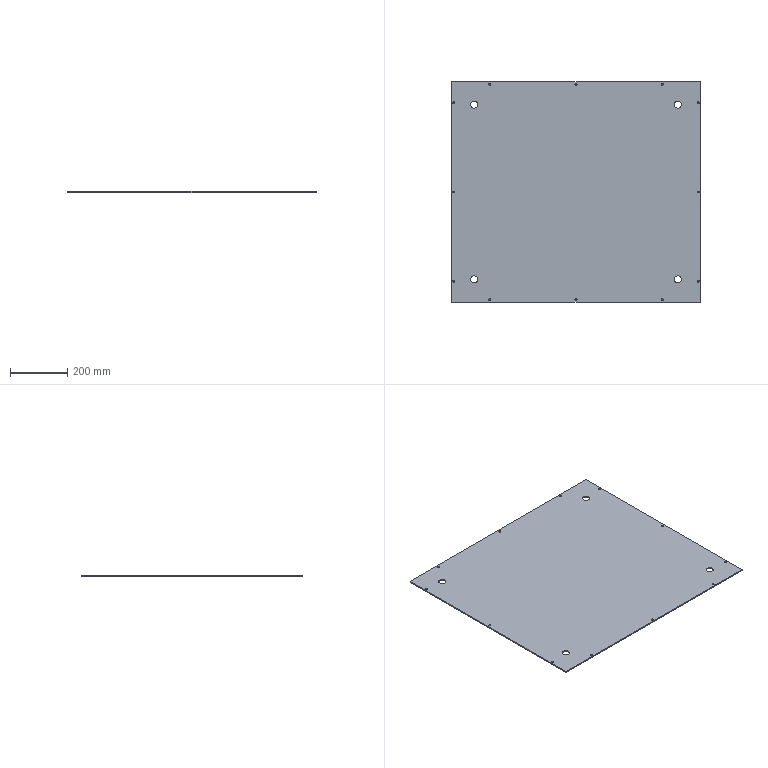Part | SolidWorks | features MirrorPattern 4, HoleWzd 2, Extrusion 1, Fillet 1, ICE 1 | 1 solid | 42 faces | box 868 x 768 x 4 mm | volume 2656781 mm3 | cylinder 36 | plane 6 | commonest cylinder face diameters 7 x24 25 x8 4 x4
STEP:
#1=CARTESIAN_POINT('',(-366.5,304.,0.));
#2=VERTEX_POINT('',#1);
#3=CARTESIAN_POINT('',(-341.5,304.,0.));
#4=VERTEX_POINT('',#3);
#5=CARTESIAN_POINT('',(-354.,304.,0.));
#6=DIRECTION('',(0.,0.,1.));
#7=DIRECTION('',(1.,0.,0.));
#8=AXIS2_PLACEMENT_3D('',#5,#6,#7);
#9=CIRCLE('',#8,12.5);
#10=EDGE_CURVE('',#2,#4,#9,.T.);
#11=ORIENTED_EDGE('',*,*,#10,.F.);
#12=CARTESIAN_POINT('',(-366.5,304.,4.));
#13=VERTEX_POINT('',#12);
#14=CARTESIAN_POINT('',(-366.5,304.,-0.001));
#15=DIRECTION('',(0.,0.,1.));
#16=VECTOR('',#15,1000.);
#17=LINE('',#14,#16);
#18=EDGE_CURVE('',#2,#13,#17,.T.);
#19=ORIENTED_EDGE('',*,*,#18,.T.);
#20=CARTESIAN_POINT('',(-341.5,304.,4.));
#21=VERTEX_POINT('',#20);
#22=CARTESIAN_POINT('',(-354.,304.,4.));
#23=DIRECTION('',(0.,0.,-1.));
#24=DIRECTION('',(1.,0.,0.));
#25=AXIS2_PLACEMENT_3D('',#22,#23,#24);
#26=CIRCLE('',#25,12.5);
#27=EDGE_CURVE('',#21,#13,#26,.T.);
#28=ORIENTED_EDGE('',*,*,#27,.F.);
#29=CARTESIAN_POINT('',(-341.5,304.,-0.001));
#30=DIRECTION('',(0.,0.,1.));
#31=VECTOR('',#30,1000.);
#32=LINE('',#29,#31);
#33=EDGE_CURVE('',#4,#21,#32,.T.);
#34=ORIENTED_EDGE('',*,*,#33,.F.);
#35=EDGE_LOOP('',(#11,#19,#28,#34));
#36=FACE_OUTER_BOUND('',#35,.T.);
#37=CARTESIAN_POINT('',(-354.,304.,-0.001));
#38=DIRECTION('',(0.,0.,1.));
#39=DIRECTION('',(1.,0.,0.));
#40=AXIS2_PLACEMENT_3D('',#37,#38,#39);
#41=CYLINDRICAL_SURFACE('',#40,12.5);
#42=ADVANCED_FACE('',(#36),#41,.F.);
#43=CARTESIAN_POINT('',(366.5,304.,0.));
#44=VERTEX_POINT('',#43);
#45=CARTESIAN_POINT('',(341.5,304.,0.));
#46=VERTEX_POINT('',#45);
#47=CARTESIAN_POINT('',(354.,304.,0.));
#48=DIRECTION('',(0.,0.,-1.));
#49=DIRECTION('',(1.,0.,0.));
#50=AXIS2_PLACEMENT_3D('',#47,#48,#49);
#51=CIRCLE('',#50,12.5);
#52=EDGE_CURVE('',#44,#46,#51,.T.);
#53=ORIENTED_EDGE('',*,*,#52,.T.);
#54=CARTESIAN_POINT('',(341.5,304.,4.));
#55=VERTEX_POINT('',#54);
#56=CARTESIAN_POINT('',(341.5,304.,-0.001));
#57=DIRECTION('',(0.,0.,1.));
#58=VECTOR('',#57,1000.);
#59=LINE('',#56,#58);
#60=EDGE_CURVE('',#46,#55,#59,.T.);
#61=ORIENTED_EDGE('',*,*,#60,.T.);
#62=CARTESIAN_POINT('',(366.5,304.,4.));
#63=VERTEX_POINT('',#62);
#64=CARTESIAN_POINT('',(354.,304.,4.));
#65=DIRECTION('',(0.,0.,1.));
#66=DIRECTION('',(-1.,0.,0.));
#67=AXIS2_PLACEMENT_3D('',#64,#65,#66);
#68=CIRCLE('',#67,12.5);
#69=EDGE_CURVE('',#55,#63,#68,.T.);
#70=ORIENTED_EDGE('',*,*,#69,.T.);
#71=CARTESIAN_POINT('',(366.5,304.,-0.001));
#72=DIRECTION('',(0.,0.,1.));
#73=VECTOR('',#72,1000.);
#74=LINE('',#71,#73);
#75=EDGE_CURVE('',#44,#63,#74,.T.);
#76=ORIENTED_EDGE('',*,*,#75,.F.);
#77=EDGE_LOOP('',(#53,#61,#70,#76));
#78=FACE_OUTER_BOUND('',#77,.T.);
#79=CARTESIAN_POINT('',(354.,304.,-0.001));
#80=DIRECTION('',(0.,0.,1.));
#81=DIRECTION('',(1.,0.,0.));
#82=AXIS2_PLACEMENT_3D('',#79,#80,#81);
#83=CYLINDRICAL_SURFACE('',#82,12.5);
#84=ADVANCED_FACE('',(#78),#83,.F.);
#85=CARTESIAN_POINT('',(341.5,-304.,0.));
#86=VERTEX_POINT('',#85);
#87=CARTESIAN_POINT('',(366.5,-304.,0.));
#88=VERTEX_POINT('',#87);
#89=CARTESIAN_POINT('',(354.,-304.,0.));
#90=DIRECTION('',(0.,0.,1.));
#91=DIRECTION('',(1.,0.,0.));
#92=AXIS2_PLACEMENT_3D('',#89,#90,#91);
#93=CIRCLE('',#92,12.5);
#94=EDGE_CURVE('',#86,#88,#93,.T.);
#95=ORIENTED_EDGE('',*,*,#94,.F.);
#96=CARTESIAN_POINT('',(341.5,-304.,4.));
#97=VERTEX_POINT('',#96);
#98=CARTESIAN_POINT('',(341.5,-304.,-0.001));
#99=DIRECTION('',(0.,0.,1.));
#100=VECTOR('',#99,1000.);
#101=LINE('',#98,#100);
#102=EDGE_CURVE('',#86,#97,#101,.T.);
#103=ORIENTED_EDGE('',*,*,#102,.T.);
#104=CARTESIAN_POINT('',(366.5,-304.,4.));
#105=VERTEX_POINT('',#104);
#106=CARTESIAN_POINT('',(354.,-304.,4.));
#107=DIRECTION('',(0.,0.,-1.));
#108=DIRECTION('',(-1.,0.,0.));
#109=AXIS2_PLACEMENT_3D('',#106,#107,#108);
#110=CIRCLE('',#109,12.5);
#111=EDGE_CURVE('',#105,#97,#110,.T.);
#112=ORIENTED_EDGE('',*,*,#111,.F.);
#113=CARTESIAN_POINT('',(366.5,-304.,-0.001));
#114=DIRECTION('',(0.,0.,1.));
#115=VECTOR('',#114,1000.);
#116=LINE('',#113,#115);
#117=EDGE_CURVE('',#88,#105,#116,.T.);
#118=ORIENTED_EDGE('',*,*,#117,.F.);
#119=EDGE_LOOP('',(#95,#103,#112,#118));
#120=FACE_OUTER_BOUND('',#119,.T.);
#121=CARTESIAN_POINT('',(354.,-304.,-0.001));
#122=DIRECTION('',(0.,0.,1.));
#123=DIRECTION('',(1.,0.,0.));
#124=AXIS2_PLACEMENT_3D('',#121,#122,#123);
#125=CYLINDRICAL_SURFACE('',#124,12.5);
#126=ADVANCED_FACE('',(#120),#125,.F.);
#127=CARTESIAN_POINT('',(-341.5,-304.,0.));
#128=VERTEX_POINT('',#127);
#129=CARTESIAN_POINT('',(-366.5,-304.,0.));
#130=VERTEX_POINT('',#129);
#131=CARTESIAN_POINT('',(-354.,-304.,0.));
#132=DIRECTION('',(0.,0.,-1.));
#133=DIRECTION('',(1.,0.,0.));
#134=AXIS2_PLACEMENT_3D('',#131,#132,#133);
#135=CIRCLE('',#134,12.5);
#136=EDGE_CURVE('',#128,#130,#135,.T.);
#137=ORIENTED_EDGE('',*,*,#136,.T.);
#138=CARTESIAN_POINT('',(-366.5,-304.,4.));
#139=VERTEX_POINT('',#138);
#140=CARTESIAN_POINT('',(-366.5,-304.,-0.001));
#141=DIRECTION('',(0.,0.,1.));
#142=VECTOR('',#141,1000.);
#143=LINE('',#140,#142);
#144=EDGE_CURVE('',#130,#139,#143,.T.);
#145=ORIENTED_EDGE('',*,*,#144,.T.);
#146=CARTESIAN_POINT('',(-341.5,-304.,4.));
#147=VERTEX_POINT('',#146);
#148=CARTESIAN_POINT('',(-354.,-304.,4.));
#149=DIRECTION('',(0.,0.,1.));
#150=DIRECTION('',(1.,0.,0.));
#151=AXIS2_PLACEMENT_3D('',#148,#149,#150);
#152=CIRCLE('',#151,12.5);
#153=EDGE_CURVE('',#139,#147,#152,.T.);
#154=ORIENTED_EDGE('',*,*,#153,.T.);
#155=CARTESIAN_POINT('',(-341.5,-304.,-0.001));
#156=DIRECTION('',(0.,0.,1.));
#157=VECTOR('',#156,1000.);
#158=LINE('',#155,#157);
#159=EDGE_CURVE('',#128,#147,#158,.T.);
#160=ORIENTED_EDGE('',*,*,#159,.F.);
#161=EDGE_LOOP('',(#137,#145,#154,#160));
#162=FACE_OUTER_BOUND('',#161,.T.);
#163=CARTESIAN_POINT('',(-354.,-304.,-0.001));
#164=DIRECTION('',(0.,0.,1.));
#165=DIRECTION('',(1.,0.,0.));
#166=AXIS2_PLACEMENT_3D('',#163,#164,#165);
#167=CYLINDRICAL_SURFACE('',#166,12.5);
#168=ADVANCED_FACE('',(#162),#167,.F.);
#169=CARTESIAN_POINT('',(-303.5,-375.,0.));
#170=VERTEX_POINT('',#169);
#171=CARTESIAN_POINT('',(-296.5,-375.,0.));
#172=VERTEX_POINT('',#171);
#173=CARTESIAN_POINT('',(-300.,-375.,0.));
#174=DIRECTION('',(0.,0.,1.));
#175=DIRECTION('',(1.,0.,0.));
#176=AXIS2_PLACEMENT_3D('',#173,#174,#175);
#177=CIRCLE('',#176,3.5);
#178=EDGE_CURVE('',#170,#172,#177,.T.);
#179=ORIENTED_EDGE('',*,*,#178,.F.);
#180=CARTESIAN_POINT('',(-303.5,-375.,4.));
#181=VERTEX_POINT('',#180);
#182=CARTESIAN_POINT('',(-303.5,-375.,4.));
#183=DIRECTION('',(0.,0.,1.));
#184=VECTOR('',#183,1000.);
#185=LINE('',#182,#184);
#186=EDGE_CURVE('',#170,#181,#185,.T.);
#187=ORIENTED_EDGE('',*,*,#186,.T.);
#188=CARTESIAN_POINT('',(-296.5,-375.,4.));
#189=VERTEX_POINT('',#188);
#190=CARTESIAN_POINT('',(-300.,-375.,4.));
#191=DIRECTION('',(0.,0.,1.));
#192=DIRECTION('',(1.,0.,0.));
#193=AXIS2_PLACEMENT_3D('',#190,#191,#192);
#194=CIRCLE('',#193,3.5);
#195=EDGE_CURVE('',#181,#189,#194,.T.);
#196=ORIENTED_EDGE('',*,*,#195,.T.);
#197=CARTESIAN_POINT('',(-296.5,-375.,4.));
#198=DIRECTION('',(0.,0.,1.));
#199=VECTOR('',#198,1000.);
#200=LINE('',#197,#199);
#201=EDGE_CURVE('',#172,#189,#200,.T.);
#202=ORIENTED_EDGE('',*,*,#201,.F.);
#203=EDGE_LOOP('',(#179,#187,#196,#202));
#204=FACE_OUTER_BOUND('',#203,.T.);
#205=CARTESIAN_POINT('',(-300.,-375.,4.));
#206=DIRECTION('',(0.,0.,1.));
#207=DIRECTION('',(1.,0.,0.));
#208=AXIS2_PLACEMENT_3D('',#205,#206,#207);
#209=CYLINDRICAL_SURFACE('',#208,3.5);
#210=ADVANCED_FACE('',(#204),#209,.F.);
#211=CARTESIAN_POINT('',(296.5,-375.,0.));
#212=VERTEX_POINT('',#211);
#213=CARTESIAN_POINT('',(303.5,-375.,0.));
#214=VERTEX_POINT('',#213);
#215=CARTESIAN_POINT('',(300.,-375.,0.));
#216=DIRECTION('',(0.,0.,1.));
#217=DIRECTION('',(1.,0.,0.));
#218=AXIS2_PLACEMENT_3D('',#215,#216,#217);
#219=CIRCLE('',#218,3.5);
#220=EDGE_CURVE('',#212,#214,#219,.T.);
#221=ORIENTED_EDGE('',*,*,#220,.F.);
#222=CARTESIAN_POINT('',(296.5,-375.,4.));
#223=VERTEX_POINT('',#222);
#224=CARTESIAN_POINT('',(296.5,-375.,4.));
#225=DIRECTION('',(0.,0.,1.));
#226=VECTOR('',#225,1000.);
#227=LINE('',#224,#226);
#228=EDGE_CURVE('',#212,#223,#227,.T.);
#229=ORIENTED_EDGE('',*,*,#228,.T.);
#230=CARTESIAN_POINT('',(303.5,-375.,4.));
#231=VERTEX_POINT('',#230);
#232=CARTESIAN_POINT('',(300.,-375.,4.));
#233=DIRECTION('',(0.,0.,1.));
#234=DIRECTION('',(1.,0.,0.));
#235=AXIS2_PLACEMENT_3D('',#232,#233,#234);
#236=CIRCLE('',#235,3.5);
#237=EDGE_CURVE('',#223,#231,#236,.T.);
#238=ORIENTED_EDGE('',*,*,#237,.T.);
#239=CARTESIAN_POINT('',(303.5,-375.,4.));
#240=DIRECTION('',(0.,0.,1.));
#241=VECTOR('',#240,1000.);
#242=LINE('',#239,#241);
#243=EDGE_CURVE('',#214,#231,#242,.T.);
#244=ORIENTED_EDGE('',*,*,#243,.F.);
#245=EDGE_LOOP('',(#221,#229,#238,#244));
#246=FACE_OUTER_BOUND('',#245,.T.);
#247=CARTESIAN_POINT('',(300.,-375.,4.));
#248=DIRECTION('',(0.,0.,1.));
#249=DIRECTION('',(1.,0.,0.));
#250=AXIS2_PLACEMENT_3D('',#247,#248,#249);
#251=CYLINDRICAL_SURFACE('',#250,3.5);
#252=ADVANCED_FACE('',(#246),#251,.F.);
#253=CARTESIAN_POINT('',(-3.5,-375.,0.));
#254=VERTEX_POINT('',#253);
#255=CARTESIAN_POINT('',(3.5,-375.,0.));
#256=VERTEX_POINT('',#255);
#257=CARTESIAN_POINT('',(0.,-375.,0.));
#258=DIRECTION('',(0.,0.,1.));
#259=DIRECTION('',(1.,0.,0.));
#260=AXIS2_PLACEMENT_3D('',#257,#258,#259);
#261=CIRCLE('',#260,3.5);
#262=EDGE_CURVE('',#254,#256,#261,.T.);
#263=ORIENTED_EDGE('',*,*,#262,.F.);
#264=CARTESIAN_POINT('',(-3.5,-375.,4.));
#265=VERTEX_POINT('',#264);
#266=CARTESIAN_POINT('',(-3.5,-375.,4.));
#267=DIRECTION('',(0.,0.,1.));
#268=VECTOR('',#267,1000.);
#269=LINE('',#266,#268);
#270=EDGE_CURVE('',#254,#265,#269,.T.);
#271=ORIENTED_EDGE('',*,*,#270,.T.);
#272=CARTESIAN_POINT('',(3.5,-375.,4.));
#273=VERTEX_POINT('',#272);
#274=CARTESIAN_POINT('',(0.,-375.,4.));
#275=DIRECTION('',(0.,0.,1.));
#276=DIRECTION('',(1.,0.,0.));
#277=AXIS2_PLACEMENT_3D('',#274,#275,#276);
#278=CIRCLE('',#277,3.5);
#279=EDGE_CURVE('',#265,#273,#278,.T.);
#280=ORIENTED_EDGE('',*,*,#279,.T.);
#281=CARTESIAN_POINT('',(3.5,-375.,4.));
#282=DIRECTION('',(0.,0.,1.));
#283=VECTOR('',#282,1000.);
#284=LINE('',#281,#283);
#285=EDGE_CURVE('',#256,#273,#284,.T.);
#286=ORIENTED_EDGE('',*,*,#285,.F.);
#287=EDGE_LOOP('',(#263,#271,#280,#286));
#288=FACE_OUTER_BOUND('',#287,.T.);
#289=CARTESIAN_POINT('',(0.,-375.,4.));
#290=DIRECTION('',(0.,0.,1.));
#291=DIRECTION('',(1.,0.,0.));
#292=AXIS2_PLACEMENT_3D('',#289,#290,#291);
#293=CYLINDRICAL_SURFACE('',#292,3.5);
#294=ADVANCED_FACE('',(#288),#293,.F.);
#295=CARTESIAN_POINT('',(-303.5,375.,0.));
#296=VERTEX_POINT('',#295);
#297=CARTESIAN_POINT('',(-296.5,375.,0.));
#298=VERTEX_POINT('',#297);
#299=CARTESIAN_POINT('',(-300.,375.,0.));
#300=DIRECTION('',(0.,0.,1.));
#301=DIRECTION('',(1.,0.,0.));
#302=AXIS2_PLACEMENT_3D('',#299,#300,#301);
#303=CIRCLE('',#302,3.5);
#304=EDGE_CURVE('',#296,#298,#303,.T.);
#305=ORIENTED_EDGE('',*,*,#304,.F.);
#306=CARTESIAN_POINT('',(-303.5,375.,4.));
#307=VERTEX_POINT('',#306);
#308=CARTESIAN_POINT('',(-303.5,375.,4.));
#309=DIRECTION('',(0.,0.,1.));
#310=VECTOR('',#309,1000.);
#311=LINE('',#308,#310);
#312=EDGE_CURVE('',#296,#307,#311,.T.);
#313=ORIENTED_EDGE('',*,*,#312,.T.);
#314=CARTESIAN_POINT('',(-296.5,375.,4.));
#315=VERTEX_POINT('',#314);
#316=CARTESIAN_POINT('',(-300.,375.,4.));
#317=DIRECTION('',(0.,0.,1.));
#318=DIRECTION('',(1.,0.,0.));
#319=AXIS2_PLACEMENT_3D('',#316,#317,#318);
#320=CIRCLE('',#319,3.5);
#321=EDGE_CURVE('',#307,#315,#320,.T.);
#322=ORIENTED_EDGE('',*,*,#321,.T.);
#323=CARTESIAN_POINT('',(-296.5,375.,4.));
#324=DIRECTION('',(0.,0.,1.));
#325=VECTOR('',#324,1000.);
#326=LINE('',#323,#325);
#327=EDGE_CURVE('',#298,#315,#326,.T.);
#328=ORIENTED_EDGE('',*,*,#327,.F.);
#329=EDGE_LOOP('',(#305,#313,#322,#328));
#330=FACE_OUTER_BOUND('',#329,.T.);
#331=CARTESIAN_POINT('',(-300.,375.,4.));
#332=DIRECTION('',(0.,0.,1.));
#333=DIRECTION('',(1.,0.,0.));
#334=AXIS2_PLACEMENT_3D('',#331,#332,#333);
#335=CYLINDRICAL_SURFACE('',#334,3.5);
#336=ADVANCED_FACE('',(#330),#335,.F.);
#337=CARTESIAN_POINT('',(296.5,375.,0.));
#338=VERTEX_POINT('',#337);
#339=CARTESIAN_POINT('',(303.5,375.,0.));
#340=VERTEX_POINT('',#339);
#341=CARTESIAN_POINT('',(300.,375.,0.));
#342=DIRECTION('',(0.,0.,1.));
#343=DIRECTION('',(1.,0.,0.));
#344=AXIS2_PLACEMENT_3D('',#341,#342,#343);
#345=CIRCLE('',#344,3.5);
#346=EDGE_CURVE('',#338,#340,#345,.T.);
#347=ORIENTED_EDGE('',*,*,#346,.F.);
#348=CARTESIAN_POINT('',(296.5,375.,4.));
#349=VERTEX_POINT('',#348);
#350=CARTESIAN_POINT('',(296.5,375.,4.));
#351=DIRECTION('',(0.,0.,1.));
#352=VECTOR('',#351,1000.);
#353=LINE('',#350,#352);
#354=EDGE_CURVE('',#338,#349,#353,.T.);
#355=ORIENTED_EDGE('',*,*,#354,.T.);
#356=CARTESIAN_POINT('',(303.5,375.,4.));
#357=VERTEX_POINT('',#356);
#358=CARTESIAN_POINT('',(300.,375.,4.));
#359=DIRECTION('',(0.,0.,1.));
#360=DIRECTION('',(1.,0.,0.));
#361=AXIS2_PLACEMENT_3D('',#358,#359,#360);
#362=CIRCLE('',#361,3.5);
#363=EDGE_CURVE('',#349,#357,#362,.T.);
#364=ORIENTED_EDGE('',*,*,#363,.T.);
#365=CARTESIAN_POINT('',(303.5,375.,4.));
#366=DIRECTION('',(0.,0.,1.));
#367=VECTOR('',#366,1000.);
#368=LINE('',#365,#367);
#369=EDGE_CURVE('',#340,#357,#368,.T.);
#370=ORIENTED_EDGE('',*,*,#369,.F.);
#371=EDGE_LOOP('',(#347,#355,#364,#370));
#372=FACE_OUTER_BOUND('',#371,.T.);
#373=CARTESIAN_POINT('',(300.,375.,4.));
#374=DIRECTION('',(0.,0.,1.));
#375=DIRECTION('',(1.,0.,0.));
#376=AXIS2_PLACEMENT_3D('',#373,#374,#375);
#377=CYLINDRICAL_SURFACE('',#376,3.5);
#378=ADVANCED_FACE('',(#372),#377,.F.);
#379=CARTESIAN_POINT('',(-3.5,375.,0.));
#380=VERTEX_POINT('',#379);
#381=CARTESIAN_POINT('',(3.5,375.,0.));
#382=VERTEX_POINT('',#381);
#383=CARTESIAN_POINT('',(0.,375.,0.));
#384=DIRECTION('',(0.,0.,1.));
#385=DIRECTION('',(1.,0.,0.));
#386=AXIS2_PLACEMENT_3D('',#383,#384,#385);
#387=CIRCLE('',#386,3.5);
#388=EDGE_CURVE('',#380,#382,#387,.T.);
#389=ORIENTED_EDGE('',*,*,#388,.F.);
#390=CARTESIAN_POINT('',(-3.5,375.,4.));
#391=VERTEX_POINT('',#390);
#392=CARTESIAN_POINT('',(-3.5,375.,4.));
#393=DIRECTION('',(0.,0.,1.));
#394=VECTOR('',#393,1000.);
#395=LINE('',#392,#394);
#396=EDGE_CURVE('',#380,#391,#395,.T.);
#397=ORIENTED_EDGE('',*,*,#396,.T.);
#398=CARTESIAN_POINT('',(3.5,375.,4.));
#399=VERTEX_POINT('',#398);
#400=CARTESIAN_POINT('',(0.,375.,4.));
#401=DIRECTION('',(0.,0.,1.));
#402=DIRECTION('',(1.,0.,0.));
#403=AXIS2_PLACEMENT_3D('',#400,#401,#402);
#404=CIRCLE('',#403,3.5);
#405=EDGE_CURVE('',#391,#399,#404,.T.);
#406=ORIENTED_EDGE('',*,*,#405,.T.);
#407=CARTESIAN_POINT('',(3.5,375.,4.));
#408=DIRECTION('',(0.,0.,1.));
#409=VECTOR('',#408,1000.);
#410=LINE('',#407,#409);
#411=EDGE_CURVE('',#382,#399,#410,.T.);
#412=ORIENTED_EDGE('',*,*,#411,.F.);
#413=EDGE_LOOP('',(#389,#397,#406,#412));
#414=FACE_OUTER_BOUND('',#413,.T.);
#415=CARTESIAN_POINT('',(0.,375.,4.));
#416=DIRECTION('',(0.,0.,1.));
#417=DIRECTION('',(1.,0.,0.));
#418=AXIS2_PLACEMENT_3D('',#415,#416,#417);
#419=CYLINDRICAL_SURFACE('',#418,3.5);
#420=ADVANCED_FACE('',(#414),#419,.F.);
#421=CARTESIAN_POINT('',(421.5,310.,0.));
#422=VERTEX_POINT('',#421);
#423=CARTESIAN_POINT('',(428.5,310.,0.));
#424=VERTEX_POINT('',#423);
#425=CARTESIAN_POINT('',(425.,310.,0.));
#426=DIRECTION('',(0.,0.,1.));
#427=DIRECTION('',(1.,0.,0.));
#428=AXIS2_PLACEMENT_3D('',#425,#426,#427);
#429=CIRCLE('',#428,3.5);
#430=EDGE_CURVE('',#422,#424,#429,.T.);
#431=ORIENTED_EDGE('',*,*,#430,.F.);
#432=CARTESIAN_POINT('',(421.5,310.,4.));
#433=VERTEX_POINT('',#432);
#434=CARTESIAN_POINT('',(421.5,310.,4.));
#435=DIRECTION('',(0.,0.,1.));
#436=VECTOR('',#435,1000.);
#437=LINE('',#434,#436);
#438=EDGE_CURVE('',#422,#433,#437,.T.);
#439=ORIENTED_EDGE('',*,*,#438,.T.);
#440=CARTESIAN_POINT('',(428.5,310.,4.));
#441=VERTEX_POINT('',#440);
#442=CARTESIAN_POINT('',(425.,310.,4.));
#443=DIRECTION('',(0.,0.,1.));
#444=DIRECTION('',(1.,0.,0.));
#445=AXIS2_PLACEMENT_3D('',#442,#443,#444);
#446=CIRCLE('',#445,3.5);
#447=EDGE_CURVE('',#433,#441,#446,.T.);
#448=ORIENTED_EDGE('',*,*,#447,.T.);
#449=CARTESIAN_POINT('',(428.5,310.,4.));
#450=DIRECTION('',(0.,0.,1.));
#451=VECTOR('',#450,1000.);
#452=LINE('',#449,#451);
#453=EDGE_CURVE('',#424,#441,#452,.T.);
#454=ORIENTED_EDGE('',*,*,#453,.F.);
#455=EDGE_LOOP('',(#431,#439,#448,#454));
#456=FACE_OUTER_BOUND('',#455,.T.);
#457=CARTESIAN_POINT('',(425.,310.,4.));
#458=DIRECTION('',(0.,0.,1.));
#459=DIRECTION('',(1.,0.,0.));
#460=AXIS2_PLACEMENT_3D('',#457,#458,#459);
#461=CYLINDRICAL_SURFACE('',#460,3.5);
#462=ADVANCED_FACE('',(#456),#461,.F.);
#463=CARTESIAN_POINT('',(421.5,-310.,0.));
#464=VERTEX_POINT('',#463);
#465=CARTESIAN_POINT('',(428.5,-310.,0.));
#466=VERTEX_POINT('',#465);
#467=CARTESIAN_POINT('',(425.,-310.,0.));
#468=DIRECTION('',(0.,0.,1.));
#469=DIRECTION('',(1.,0.,0.));
#470=AXIS2_PLACEMENT_3D('',#467,#468,#469);
#471=CIRCLE('',#470,3.5);
#472=EDGE_CURVE('',#464,#466,#471,.T.);
#473=ORIENTED_EDGE('',*,*,#472,.F.);
#474=CARTESIAN_POINT('',(421.5,-310.,4.));
#475=VERTEX_POINT('',#474);
#476=CARTESIAN_POINT('',(421.5,-310.,4.));
#477=DIRECTION('',(0.,0.,1.));
#478=VECTOR('',#477,1000.);
#479=LINE('',#476,#478);
#480=EDGE_CURVE('',#464,#475,#479,.T.);
#481=ORIENTED_EDGE('',*,*,#480,.T.);
#482=CARTESIAN_POINT('',(428.5,-310.,4.));
#483=VERTEX_POINT('',#482);
#484=CARTESIAN_POINT('',(425.,-310.,4.));
#485=DIRECTION('',(0.,0.,1.));
#486=DIRECTION('',(1.,0.,0.));
#487=AXIS2_PLACEMENT_3D('',#484,#485,#486);
#488=CIRCLE('',#487,3.5);
#489=EDGE_CURVE('',#475,#483,#488,.T.);
#490=ORIENTED_EDGE('',*,*,#489,.T.);
#491=CARTESIAN_POINT('',(428.5,-310.,4.));
#492=DIRECTION('',(0.,0.,1.));
#493=VECTOR('',#492,1000.);
#494=LINE('',#491,#493);
#495=EDGE_CURVE('',#466,#483,#494,.T.);
#496=ORIENTED_EDGE('',*,*,#495,.F.);
#497=EDGE_LOOP('',(#473,#481,#490,#496));
#498=FACE_OUTER_BOUND('',#497,.T.);
#499=CARTESIAN_POINT('',(425.,-310.,4.));
#500=DIRECTION('',(0.,0.,1.));
#501=DIRECTION('',(1.,0.,0.));
#502=AXIS2_PLACEMENT_3D('',#499,#500,#501);
#503=CYLINDRICAL_SURFACE('',#502,3.5);
#504=ADVANCED_FACE('',(#498),#503,.F.);
#505=CARTESIAN_POINT('',(421.5,0.,0.));
#506=VERTEX_POINT('',#505);
#507=CARTESIAN_POINT('',(428.5,0.,0.));
#508=VERTEX_POINT('',#507);
#509=CARTESIAN_POINT('',(425.,0.,0.));
#510=DIRECTION('',(0.,0.,1.));
#511=DIRECTION('',(1.,0.,0.));
#512=AXIS2_PLACEMENT_3D('',#509,#510,#511);
#513=CIRCLE('',#512,3.5);
#514=EDGE_CURVE('',#506,#508,#513,.T.);
#515=ORIENTED_EDGE('',*,*,#514,.F.);
#516=CARTESIAN_POINT('',(421.5,0.,4.));
#517=VERTEX_POINT('',#516);
#518=CARTESIAN_POINT('',(421.5,0.,4.));
#519=DIRECTION('',(0.,0.,1.));
#520=VECTOR('',#519,1000.);
#521=LINE('',#518,#520);
#522=EDGE_CURVE('',#506,#517,#521,.T.);
#523=ORIENTED_EDGE('',*,*,#522,.T.);
#524=CARTESIAN_POINT('',(428.5,0.,4.));
#525=VERTEX_POINT('',#524);
#526=CARTESIAN_POINT('',(425.,0.,4.));
#527=DIRECTION('',(0.,0.,1.));
#528=DIRECTION('',(1.,0.,0.));
#529=AXIS2_PLACEMENT_3D('',#526,#527,#528);
#530=CIRCLE('',#529,3.5);
#531=EDGE_CURVE('',#517,#525,#530,.T.);
#532=ORIENTED_EDGE('',*,*,#531,.T.);
#533=CARTESIAN_POINT('',(428.5,0.,4.));
#534=DIRECTION('',(0.,0.,1.));
#535=VECTOR('',#534,1000.);
#536=LINE('',#533,#535);
#537=EDGE_CURVE('',#508,#525,#536,.T.);
#538=ORIENTED_EDGE('',*,*,#537,.F.);
#539=EDGE_LOOP('',(#515,#523,#532,#538));
#540=FACE_OUTER_BOUND('',#539,.T.);
#541=CARTESIAN_POINT('',(425.,0.,4.));
#542=DIRECTION('',(0.,0.,1.));
#543=DIRECTION('',(1.,0.,0.));
#544=AXIS2_PLACEMENT_3D('',#541,#542,#543);
#545=CYLINDRICAL_SURFACE('',#544,3.5);
#546=ADVANCED_FACE('',(#540),#545,.F.);
#547=CARTESIAN_POINT('',(-428.5,310.,0.));
#548=VERTEX_POINT('',#547);
#549=CARTESIAN_POINT('',(-421.5,310.,0.));
#550=VERTEX_POINT('',#549);
#551=CARTESIAN_POINT('',(-425.,310.,0.));
#552=DIRECTION('',(0.,0.,1.));
#553=DIRECTION('',(1.,0.,0.));
#554=AXIS2_PLACEMENT_3D('',#551,#552,#553);
#555=CIRCLE('',#554,3.5);
#556=EDGE_CURVE('',#548,#550,#555,.T.);
#557=ORIENTED_EDGE('',*,*,#556,.F.);
#558=CARTESIAN_POINT('',(-428.5,310.,4.));
#559=VERTEX_POINT('',#558);
#560=CARTESIAN_POINT('',(-428.5,310.,4.));
#561=DIRECTION('',(0.,0.,1.));
#562=VECTOR('',#561,1000.);
#563=LINE('',#560,#562);
#564=EDGE_CURVE('',#548,#559,#563,.T.);
#565=ORIENTED_EDGE('',*,*,#564,.T.);
#566=CARTESIAN_POINT('',(-421.5,310.,4.));
#567=VERTEX_POINT('',#566);
#568=CARTESIAN_POINT('',(-425.,310.,4.));
#569=DIRECTION('',(0.,0.,1.));
#570=DIRECTION('',(1.,0.,0.));
#571=AXIS2_PLACEMENT_3D('',#568,#569,#570);
#572=CIRCLE('',#571,3.5);
#573=EDGE_CURVE('',#559,#567,#572,.T.);
#574=ORIENTED_EDGE('',*,*,#573,.T.);
#575=CARTESIAN_POINT('',(-421.5,310.,4.));
#576=DIRECTION('',(0.,0.,1.));
#577=VECTOR('',#576,1000.);
#578=LINE('',#575,#577);
#579=EDGE_CURVE('',#550,#567,#578,.T.);
#580=ORIENTED_EDGE('',*,*,#579,.F.);
#581=EDGE_LOOP('',(#557,#565,#574,#580));
#582=FACE_OUTER_BOUND('',#581,.T.);
#583=CARTESIAN_POINT('',(-425.,310.,4.));
#584=DIRECTION('',(0.,0.,1.));
#585=DIRECTION('',(1.,0.,0.));
#586=AXIS2_PLACEMENT_3D('',#583,#584,#585);
#587=CYLINDRICAL_SURFACE('',#586,3.5);
#588=ADVANCED_FACE('',(#582),#587,.F.);
#589=CARTESIAN_POINT('',(-428.5,-310.,0.));
#590=VERTEX_POINT('',#589);
#591=CARTESIAN_POINT('',(-421.5,-310.,0.));
#592=VERTEX_POINT('',#591);
#593=CARTESIAN_POINT('',(-425.,-310.,0.));
#594=DIRECTION('',(0.,0.,1.));
#595=DIRECTION('',(1.,0.,0.));
#596=AXIS2_PLACEMENT_3D('',#593,#594,#595);
#597=CIRCLE('',#596,3.5);
#598=EDGE_CURVE('',#590,#592,#597,.T.);
#599=ORIENTED_EDGE('',*,*,#598,.F.);
#600=CARTESIAN_POINT('',(-428.5,-310.,4.));
#601=VERTEX_POINT('',#600);
#602=CARTESIAN_POINT('',(-428.5,-310.,4.));
#603=DIRECTION('',(0.,0.,1.));
#604=VECTOR('',#603,1000.);
#605=LINE('',#602,#604);
#606=EDGE_CURVE('',#590,#601,#605,.T.);
#607=ORIENTED_EDGE('',*,*,#606,.T.);
#608=CARTESIAN_POINT('',(-421.5,-310.,4.));
#609=VERTEX_POINT('',#608);
#610=CARTESIAN_POINT('',(-425.,-310.,4.));
#611=DIRECTION('',(0.,0.,1.));
#612=DIRECTION('',(1.,0.,0.));
#613=AXIS2_PLACEMENT_3D('',#610,#611,#612);
#614=CIRCLE('',#613,3.5);
#615=EDGE_CURVE('',#601,#609,#614,.T.);
#616=ORIENTED_EDGE('',*,*,#615,.T.);
#617=CARTESIAN_POINT('',(-421.5,-310.,4.));
#618=DIRECTION('',(0.,0.,1.));
#619=VECTOR('',#618,1000.);
#620=LINE('',#617,#619);
#621=EDGE_CURVE('',#592,#609,#620,.T.);
#622=ORIENTED_EDGE('',*,*,#621,.F.);
#623=EDGE_LOOP('',(#599,#607,#616,#622));
#624=FACE_OUTER_BOUND('',#623,.T.);
#625=CARTESIAN_POINT('',(-425.,-310.,4.));
#626=DIRECTION('',(0.,0.,1.));
#627=DIRECTION('',(1.,0.,0.));
#628=AXIS2_PLACEMENT_3D('',#625,#626,#627);
#629=CYLINDRICAL_SURFACE('',#628,3.5);
#630=ADVANCED_FACE('',(#624),#629,.F.);
#631=CARTESIAN_POINT('',(-428.5,0.,0.));
#632=VERTEX_POINT('',#631);
#633=CARTESIAN_POINT('',(-421.5,0.,0.));
#634=VERTEX_POINT('',#633);
#635=CARTESIAN_POINT('',(-425.,0.,0.));
#636=DIRECTION('',(0.,0.,1.));
#637=DIRECTION('',(1.,0.,0.));
#638=AXIS2_PLACEMENT_3D('',#635,#636,#637);
#639=CIRCLE('',#638,3.5);
#640=EDGE_CURVE('',#632,#634,#639,.T.);
#641=ORIENTED_EDGE('',*,*,#640,.F.);
#642=CARTESIAN_POINT('',(-428.5,0.,4.));
#643=VERTEX_POINT('',#642);
#644=CARTESIAN_POINT('',(-428.5,0.,4.));
#645=DIRECTION('',(0.,0.,1.));
#646=VECTOR('',#645,1000.);
#647=LINE('',#644,#646);
#648=EDGE_CURVE('',#632,#643,#647,.T.);
#649=ORIENTED_EDGE('',*,*,#648,.T.);
#650=CARTESIAN_POINT('',(-421.5,0.,4.));
#651=VERTEX_POINT('',#650);
#652=CARTESIAN_POINT('',(-425.,0.,4.));
#653=DIRECTION('',(0.,0.,1.));
#654=DIRECTION('',(1.,0.,0.));
#655=AXIS2_PLACEMENT_3D('',#652,#653,#654);
#656=CIRCLE('',#655,3.5);
#657=EDGE_CURVE('',#643,#651,#656,.T.);
#658=ORIENTED_EDGE('',*,*,#657,.T.);
#659=CARTESIAN_POINT('',(-421.5,0.,4.));
#660=DIRECTION('',(0.,0.,1.));
#661=VECTOR('',#660,1000.);
#662=LINE('',#659,#661);
#663=EDGE_CURVE('',#634,#651,#662,.T.);
#664=ORIENTED_EDGE('',*,*,#663,.F.);
#665=EDGE_LOOP('',(#641,#649,#658,#664));
#666=FACE_OUTER_BOUND('',#665,.T.);
#667=CARTESIAN_POINT('',(-425.,0.,4.));
#668=DIRECTION('',(0.,0.,1.));
#669=DIRECTION('',(1.,0.,0.));
#670=AXIS2_PLACEMENT_3D('',#667,#668,#669);
#671=CYLINDRICAL_SURFACE('',#670,3.5);
#672=ADVANCED_FACE('',(#666),#671,.F.);
#673=CARTESIAN_POINT('',(-434.,382.,0.));
#674=VERTEX_POINT('',#673);
#675=CARTESIAN_POINT('',(-434.,-382.,0.));
#676=VERTEX_POINT('',#675);
#677=CARTESIAN_POINT('',(-434.,-384.,0.));
#678=DIRECTION('',(0.,-1.,0.));
#679=VECTOR('',#678,1000.);
#680=LINE('',#677,#679);
#681=EDGE_CURVE('',#674,#676,#680,.T.);
#682=ORIENTED_EDGE('',*,*,#681,.T.);
#683=CARTESIAN_POINT('',(-434.,-382.,4.));
#684=VERTEX_POINT('',#683);
#685=CARTESIAN_POINT('',(-434.,-382.,4.));
#686=DIRECTION('',(0.,0.,1.));
#687=VECTOR('',#686,1000.);
#688=LINE('',#685,#687);
#689=EDGE_CURVE('',#676,#684,#688,.T.);
#690=ORIENTED_EDGE('',*,*,#689,.T.);
#691=CARTESIAN_POINT('',(-434.,382.,4.));
#692=VERTEX_POINT('',#691);
#693=CARTESIAN_POINT('',(-434.,-384.,4.));
#694=DIRECTION('',(0.,-1.,0.));
#695=VECTOR('',#694,1000.);
#696=LINE('',#693,#695);
#697=EDGE_CURVE('',#692,#684,#696,.T.);
#698=ORIENTED_EDGE('',*,*,#697,.F.);
#699=CARTESIAN_POINT('',(-434.,382.,4.));
#700=DIRECTION('',(0.,0.,-1.));
#701=VECTOR('',#700,1000.);
#702=LINE('',#699,#701);
#703=EDGE_CURVE('',#692,#674,#702,.T.);
#704=ORIENTED_EDGE('',*,*,#703,.T.);
#705=EDGE_LOOP('',(#682,#690,#698,#704));
#706=FACE_OUTER_BOUND('',#705,.T.);
#707=CARTESIAN_POINT('',(-434.,-384.,4.));
#708=DIRECTION('',(1.,0.,0.));
#709=DIRECTION('',(0.,0.,-1.));
#710=AXIS2_PLACEMENT_3D('',#707,#708,#709);
#711=PLANE('',#710);
#712=ADVANCED_FACE('',(#706),#711,.F.);
#713=CARTESIAN_POINT('',(-432.,-384.,0.));
#714=VERTEX_POINT('',#713);
#715=CARTESIAN_POINT('',(432.,-384.,0.));
#716=VERTEX_POINT('',#715);
#717=CARTESIAN_POINT('',(434.,-384.,0.));
#718=DIRECTION('',(1.,0.,0.));
#719=VECTOR('',#718,1000.);
#720=LINE('',#717,#719);
#721=EDGE_CURVE('',#714,#716,#720,.T.);
#722=ORIENTED_EDGE('',*,*,#721,.T.);
#723=CARTESIAN_POINT('',(432.,-384.,4.));
#724=VERTEX_POINT('',#723);
#725=CARTESIAN_POINT('',(432.,-384.,4.));
#726=DIRECTION('',(0.,0.,1.));
#727=VECTOR('',#726,1000.);
#728=LINE('',#725,#727);
#729=EDGE_CURVE('',#716,#724,#728,.T.);
#730=ORIENTED_EDGE('',*,*,#729,.T.);
#731=CARTESIAN_POINT('',(-432.,-384.,4.));
#732=VERTEX_POINT('',#731);
#733=CARTESIAN_POINT('',(434.,-384.,4.));
#734=DIRECTION('',(1.,0.,0.));
#735=VECTOR('',#734,1000.);
#736=LINE('',#733,#735);
#737=EDGE_CURVE('',#732,#724,#736,.T.);
#738=ORIENTED_EDGE('',*,*,#737,.F.);
#739=CARTESIAN_POINT('',(-432.,-384.,4.));
#740=DIRECTION('',(0.,0.,-1.));
#741=VECTOR('',#740,1000.);
#742=LINE('',#739,#741);
#743=EDGE_CURVE('',#732,#714,#742,.T.);
#744=ORIENTED_EDGE('',*,*,#743,.T.);
#745=EDGE_LOOP('',(#722,#730,#738,#744));
#746=FACE_OUTER_BOUND('',#745,.T.);
#747=CARTESIAN_POINT('',(434.,-384.,4.));
#748=DIRECTION('',(0.,1.,0.));
#749=DIRECTION('',(-1.,0.,0.));
#750=AXIS2_PLACEMENT_3D('',#747,#748,#749);
#751=PLANE('',#750);
#752=ADVANCED_FACE('',(#746),#751,.F.);
#753=CARTESIAN_POINT('',(434.,-382.,0.));
#754=VERTEX_POINT('',#753);
#755=CARTESIAN_POINT('',(434.,382.,0.));
#756=VERTEX_POINT('',#755);
#757=CARTESIAN_POINT('',(434.,-384.,0.));
#758=DIRECTION('',(0.,1.,0.));
#759=VECTOR('',#758,1000.);
#760=LINE('',#757,#759);
#761=EDGE_CURVE('',#754,#756,#760,.T.);
#762=ORIENTED_EDGE('',*,*,#761,.T.);
#763=CARTESIAN_POINT('',(434.,382.,4.));
#764=VERTEX_POINT('',#763);
#765=CARTESIAN_POINT('',(434.,382.,4.));
#766=DIRECTION('',(0.,0.,1.));
#767=VECTOR('',#766,1000.);
#768=LINE('',#765,#767);
#769=EDGE_CURVE('',#756,#764,#768,.T.);
#770=ORIENTED_EDGE('',*,*,#769,.T.);
#771=CARTESIAN_POINT('',(434.,-382.,4.));
#772=VERTEX_POINT('',#771);
#773=CARTESIAN_POINT('',(434.,-384.,4.));
#774=DIRECTION('',(0.,1.,0.));
#775=VECTOR('',#774,1000.);
#776=LINE('',#773,#775);
#777=EDGE_CURVE('',#772,#764,#776,.T.);
#778=ORIENTED_EDGE('',*,*,#777,.F.);
#779=CARTESIAN_POINT('',(434.,-382.,4.));
#780=DIRECTION('',(0.,0.,-1.));
#781=VECTOR('',#780,1000.);
#782=LINE('',#779,#781);
#783=EDGE_CURVE('',#772,#754,#782,.T.);
#784=ORIENTED_EDGE('',*,*,#783,.T.);
#785=EDGE_LOOP('',(#762,#770,#778,#784));
#786=FACE_OUTER_BOUND('',#785,.T.);
#787=CARTESIAN_POINT('',(434.,-384.,4.));
#788=DIRECTION('',(-1.,0.,0.));
#789=DIRECTION('',(0.,-1.,0.));
#790=AXIS2_PLACEMENT_3D('',#787,#788,#789);
#791=PLANE('',#790);
#792=ADVANCED_FACE('',(#786),#791,.F.);
#793=CARTESIAN_POINT('',(432.,384.,4.));
#794=VERTEX_POINT('',#793);
#795=CARTESIAN_POINT('',(-432.,384.,4.));
#796=VERTEX_POINT('',#795);
#797=CARTESIAN_POINT('',(434.,384.,4.));
#798=DIRECTION('',(-1.,0.,0.));
#799=VECTOR('',#798,1000.);
#800=LINE('',#797,#799);
#801=EDGE_CURVE('',#794,#796,#800,.T.);
#802=ORIENTED_EDGE('',*,*,#801,.F.);
#803=CARTESIAN_POINT('',(432.,384.,0.));
#804=VERTEX_POINT('',#803);
#805=CARTESIAN_POINT('',(432.,384.,4.));
#806=DIRECTION('',(0.,0.,-1.));
#807=VECTOR('',#806,1000.);
#808=LINE('',#805,#807);
#809=EDGE_CURVE('',#794,#804,#808,.T.);
#810=ORIENTED_EDGE('',*,*,#809,.T.);
#811=CARTESIAN_POINT('',(-432.,384.,0.));
#812=VERTEX_POINT('',#811);
#813=CARTESIAN_POINT('',(434.,384.,0.));
#814=DIRECTION('',(-1.,0.,0.));
#815=VECTOR('',#814,1000.);
#816=LINE('',#813,#815);
#817=EDGE_CURVE('',#804,#812,#816,.T.);
#818=ORIENTED_EDGE('',*,*,#817,.T.);
#819=CARTESIAN_POINT('',(-432.,384.,4.));
#820=DIRECTION('',(0.,0.,1.));
#821=VECTOR('',#820,1000.);
#822=LINE('',#819,#821);
#823=EDGE_CURVE('',#812,#796,#822,.T.);
#824=ORIENTED_EDGE('',*,*,#823,.T.);
#825=EDGE_LOOP('',(#802,#810,#818,#824));
#826=FACE_OUTER_BOUND('',#825,.T.);
#827=CARTESIAN_POINT('',(434.,384.,4.));
#828=DIRECTION('',(0.,-1.,0.));
#829=DIRECTION('',(1.,0.,0.));
#830=AXIS2_PLACEMENT_3D('',#827,#828,#829);
#831=PLANE('',#830);
#832=ADVANCED_FACE('',(#826),#831,.F.);
#833=ORIENTED_EDGE('',*,*,#27,.T.);
#834=CARTESIAN_POINT('',(-354.,304.,4.));
#835=DIRECTION('',(0.,0.,-1.));
#836=DIRECTION('',(1.,0.,0.));
#837=AXIS2_PLACEMENT_3D('',#834,#835,#836);
#838=CIRCLE('',#837,12.5);
#839=EDGE_CURVE('',#13,#21,#838,.T.);
#840=ORIENTED_EDGE('',*,*,#839,.T.);
#841=EDGE_LOOP('',(#833,#840));
#842=FACE_BOUND('',#841,.T.);
#843=CARTESIAN_POINT('',(354.,304.,4.));
#844=DIRECTION('',(0.,0.,1.));
#845=DIRECTION('',(-1.,0.,0.));
#846=AXIS2_PLACEMENT_3D('',#843,#844,#845);
#847=CIRCLE('',#846,12.5);
#848=EDGE_CURVE('',#63,#55,#847,.T.);
#849=ORIENTED_EDGE('',*,*,#848,.F.);
#850=ORIENTED_EDGE('',*,*,#69,.F.);
#851=EDGE_LOOP('',(#849,#850));
#852=FACE_BOUND('',#851,.T.);
#853=ORIENTED_EDGE('',*,*,#111,.T.);
#854=CARTESIAN_POINT('',(354.,-304.,4.));
#855=DIRECTION('',(0.,0.,-1.));
#856=DIRECTION('',(-1.,0.,0.));
#857=AXIS2_PLACEMENT_3D('',#854,#855,#856);
#858=CIRCLE('',#857,12.5);
#859=EDGE_CURVE('',#97,#105,#858,.T.);
#860=ORIENTED_EDGE('',*,*,#859,.T.);
#861=EDGE_LOOP('',(#853,#860));
#862=FACE_BOUND('',#861,.T.);
#863=CARTESIAN_POINT('',(-354.,-304.,4.));
#864=DIRECTION('',(0.,0.,1.));
#865=DIRECTION('',(1.,0.,0.));
#866=AXIS2_PLACEMENT_3D('',#863,#864,#865);
#867=CIRCLE('',#866,12.5);
#868=EDGE_CURVE('',#147,#139,#867,.T.);
#869=ORIENTED_EDGE('',*,*,#868,.F.);
#870=ORIENTED_EDGE('',*,*,#153,.F.);
#871=EDGE_LOOP('',(#869,#870));
#872=FACE_BOUND('',#871,.T.);
#873=CARTESIAN_POINT('',(-300.,-375.,4.));
#874=DIRECTION('',(0.,0.,1.));
#875=DIRECTION('',(1.,0.,0.));
#876=AXIS2_PLACEMENT_3D('',#873,#874,#875);
#877=CIRCLE('',#876,3.5);
#878=EDGE_CURVE('',#189,#181,#877,.T.);
#879=ORIENTED_EDGE('',*,*,#878,.F.);
#880=ORIENTED_EDGE('',*,*,#195,.F.);
#881=EDGE_LOOP('',(#879,#880));
#882=FACE_BOUND('',#881,.T.);
#883=CARTESIAN_POINT('',(300.,-375.,4.));
#884=DIRECTION('',(0.,0.,1.));
#885=DIRECTION('',(1.,0.,0.));
#886=AXIS2_PLACEMENT_3D('',#883,#884,#885);
#887=CIRCLE('',#886,3.5);
#888=EDGE_CURVE('',#231,#223,#887,.T.);
#889=ORIENTED_EDGE('',*,*,#888,.F.);
#890=ORIENTED_EDGE('',*,*,#237,.F.);
#891=EDGE_LOOP('',(#889,#890));
#892=FACE_BOUND('',#891,.T.);
#893=CARTESIAN_POINT('',(0.,-375.,4.));
#894=DIRECTION('',(0.,0.,1.));
#895=DIRECTION('',(1.,0.,0.));
#896=AXIS2_PLACEMENT_3D('',#893,#894,#895);
#897=CIRCLE('',#896,3.5);
#898=EDGE_CURVE('',#273,#265,#897,.T.);
#899=ORIENTED_EDGE('',*,*,#898,.F.);
#900=ORIENTED_EDGE('',*,*,#279,.F.);
#901=EDGE_LOOP('',(#899,#900));
#902=FACE_BOUND('',#901,.T.);
#903=CARTESIAN_POINT('',(-300.,375.,4.));
#904=DIRECTION('',(0.,0.,1.));
#905=DIRECTION('',(1.,0.,0.));
#906=AXIS2_PLACEMENT_3D('',#903,#904,#905);
#907=CIRCLE('',#906,3.5);
#908=EDGE_CURVE('',#315,#307,#907,.T.);
#909=ORIENTED_EDGE('',*,*,#908,.F.);
#910=ORIENTED_EDGE('',*,*,#321,.F.);
#911=EDGE_LOOP('',(#909,#910));
#912=FACE_BOUND('',#911,.T.);
#913=CARTESIAN_POINT('',(300.,375.,4.));
#914=DIRECTION('',(0.,0.,1.));
#915=DIRECTION('',(1.,0.,0.));
#916=AXIS2_PLACEMENT_3D('',#913,#914,#915);
#917=CIRCLE('',#916,3.5);
#918=EDGE_CURVE('',#357,#349,#917,.T.);
#919=ORIENTED_EDGE('',*,*,#918,.F.);
#920=ORIENTED_EDGE('',*,*,#363,.F.);
#921=EDGE_LOOP('',(#919,#920));
#922=FACE_BOUND('',#921,.T.);
#923=CARTESIAN_POINT('',(0.,375.,4.));
#924=DIRECTION('',(0.,0.,1.));
#925=DIRECTION('',(1.,0.,0.));
#926=AXIS2_PLACEMENT_3D('',#923,#924,#925);
#927=CIRCLE('',#926,3.5);
#928=EDGE_CURVE('',#399,#391,#927,.T.);
#929=ORIENTED_EDGE('',*,*,#928,.F.);
#930=ORIENTED_EDGE('',*,*,#405,.F.);
#931=EDGE_LOOP('',(#929,#930));
#932=FACE_BOUND('',#931,.T.);
#933=CARTESIAN_POINT('',(425.,310.,4.));
#934=DIRECTION('',(0.,0.,1.));
#935=DIRECTION('',(1.,0.,0.));
#936=AXIS2_PLACEMENT_3D('',#933,#934,#935);
#937=CIRCLE('',#936,3.5);
#938=EDGE_CURVE('',#441,#433,#937,.T.);
#939=ORIENTED_EDGE('',*,*,#938,.F.);
#940=ORIENTED_EDGE('',*,*,#447,.F.);
#941=EDGE_LOOP('',(#939,#940));
#942=FACE_BOUND('',#941,.T.);
#943=CARTESIAN_POINT('',(425.,-310.,4.));
#944=DIRECTION('',(0.,0.,1.));
#945=DIRECTION('',(1.,0.,0.));
#946=AXIS2_PLACEMENT_3D('',#943,#944,#945);
#947=CIRCLE('',#946,3.5);
#948=EDGE_CURVE('',#483,#475,#947,.T.);
#949=ORIENTED_EDGE('',*,*,#948,.F.);
#950=ORIENTED_EDGE('',*,*,#489,.F.);
#951=EDGE_LOOP('',(#949,#950));
#952=FACE_BOUND('',#951,.T.);
#953=CARTESIAN_POINT('',(425.,0.,4.));
#954=DIRECTION('',(0.,0.,1.));
#955=DIRECTION('',(1.,0.,0.));
#956=AXIS2_PLACEMENT_3D('',#953,#954,#955);
#957=CIRCLE('',#956,3.5);
#958=EDGE_CURVE('',#525,#517,#957,.T.);
#959=ORIENTED_EDGE('',*,*,#958,.F.);
#960=ORIENTED_EDGE('',*,*,#531,.F.);
#961=EDGE_LOOP('',(#959,#960));
#962=FACE_BOUND('',#961,.T.);
#963=CARTESIAN_POINT('',(-425.,310.,4.));
#964=DIRECTION('',(0.,0.,1.));
#965=DIRECTION('',(1.,0.,0.));
#966=AXIS2_PLACEMENT_3D('',#963,#964,#965);
#967=CIRCLE('',#966,3.5);
#968=EDGE_CURVE('',#567,#559,#967,.T.);
#969=ORIENTED_EDGE('',*,*,#968,.F.);
#970=ORIENTED_EDGE('',*,*,#573,.F.);
#971=EDGE_LOOP('',(#969,#970));
#972=FACE_BOUND('',#971,.T.);
#973=CARTESIAN_POINT('',(-425.,-310.,4.));
#974=DIRECTION('',(0.,0.,1.));
#975=DIRECTION('',(1.,0.,0.));
#976=AXIS2_PLACEMENT_3D('',#973,#974,#975);
#977=CIRCLE('',#976,3.5);
#978=EDGE_CURVE('',#609,#601,#977,.T.);
#979=ORIENTED_EDGE('',*,*,#978,.F.);
#980=ORIENTED_EDGE('',*,*,#615,.F.);
#981=EDGE_LOOP('',(#979,#980));
#982=FACE_BOUND('',#981,.T.);
#983=CARTESIAN_POINT('',(-425.,0.,4.));
#984=DIRECTION('',(0.,0.,1.));
#985=DIRECTION('',(1.,0.,0.));
#986=AXIS2_PLACEMENT_3D('',#983,#984,#985);
#987=CIRCLE('',#986,3.5);
#988=EDGE_CURVE('',#651,#643,#987,.T.);
#989=ORIENTED_EDGE('',*,*,#988,.F.);
#990=ORIENTED_EDGE('',*,*,#657,.F.);
#991=EDGE_LOOP('',(#989,#990));
#992=FACE_BOUND('',#991,.T.);
#993=ORIENTED_EDGE('',*,*,#777,.T.);
#994=CARTESIAN_POINT('',(432.,382.,4.));
#995=DIRECTION('',(0.,0.,1.));
#996=DIRECTION('',(1.,0.,0.));
#997=AXIS2_PLACEMENT_3D('',#994,#995,#996);
#998=CIRCLE('',#997,2.);
#999=EDGE_CURVE('',#764,#794,#998,.T.);
#1000=ORIENTED_EDGE('',*,*,#999,.T.);
#1001=ORIENTED_EDGE('',*,*,#801,.T.);
#1002=CARTESIAN_POINT('',(-432.,382.,4.));
#1003=DIRECTION('',(0.,0.,1.));
#1004=DIRECTION('',(1.,0.,0.));
#1005=AXIS2_PLACEMENT_3D('',#1002,#1003,#1004);
#1006=CIRCLE('',#1005,2.);
#1007=EDGE_CURVE('',#796,#692,#1006,.T.);
#1008=ORIENTED_EDGE('',*,*,#1007,.T.);
#1009=ORIENTED_EDGE('',*,*,#697,.T.);
#1010=CARTESIAN_POINT('',(-432.,-382.,4.));
#1011=DIRECTION('',(0.,0.,1.));
#1012=DIRECTION('',(1.,0.,0.));
#1013=AXIS2_PLACEMENT_3D('',#1010,#1011,#1012);
#1014=CIRCLE('',#1013,2.);
#1015=EDGE_CURVE('',#684,#732,#1014,.T.);
#1016=ORIENTED_EDGE('',*,*,#1015,.T.);
#1017=ORIENTED_EDGE('',*,*,#737,.T.);
#1018=CARTESIAN_POINT('',(432.,-382.,4.));
#1019=DIRECTION('',(0.,0.,1.));
#1020=DIRECTION('',(1.,0.,0.));
#1021=AXIS2_PLACEMENT_3D('',#1018,#1019,#1020);
#1022=CIRCLE('',#1021,2.);
#1023=EDGE_CURVE('',#724,#772,#1022,.T.);
#1024=ORIENTED_EDGE('',*,*,#1023,.T.);
#1025=EDGE_LOOP('',(#993,#1000,#1001,#1008,#1009,#1016,#1017,#1024));
#1026=FACE_OUTER_BOUND('',#1025,.T.);
#1027=CARTESIAN_POINT('',(0.,0.,4.));
#1028=DIRECTION('',(0.,0.,1.));
#1029=DIRECTION('',(1.,0.,0.));
#1030=AXIS2_PLACEMENT_3D('',#1027,#1028,#1029);
#1031=PLANE('',#1030);
#1032=ADVANCED_FACE('',(#842,#852,#862,#872,#882,#892,#902,#912,#922,#932,#942,#952,#962,#972,#982,#992,#1026),#1031,.T.);
#1033=CARTESIAN_POINT('',(-354.,304.,0.));
#1034=DIRECTION('',(0.,0.,1.));
#1035=DIRECTION('',(1.,0.,0.));
#1036=AXIS2_PLACEMENT_3D('',#1033,#1034,#1035);
#1037=CIRCLE('',#1036,12.5);
#1038=EDGE_CURVE('',#4,#2,#1037,.T.);
#1039=ORIENTED_EDGE('',*,*,#1038,.T.);
#1040=ORIENTED_EDGE('',*,*,#10,.T.);
#1041=EDGE_LOOP('',(#1039,#1040));
#1042=FACE_BOUND('',#1041,.T.);
#1043=ORIENTED_EDGE('',*,*,#52,.F.);
#1044=CARTESIAN_POINT('',(354.,304.,0.));
#1045=DIRECTION('',(0.,0.,-1.));
#1046=DIRECTION('',(1.,0.,0.));
#1047=AXIS2_PLACEMENT_3D('',#1044,#1045,#1046);
#1048=CIRCLE('',#1047,12.5);
#1049=EDGE_CURVE('',#46,#44,#1048,.T.);
#1050=ORIENTED_EDGE('',*,*,#1049,.F.);
#1051=EDGE_LOOP('',(#1043,#1050));
#1052=FACE_BOUND('',#1051,.T.);
#1053=CARTESIAN_POINT('',(354.,-304.,0.));
#1054=DIRECTION('',(0.,0.,1.));
#1055=DIRECTION('',(1.,0.,0.));
#1056=AXIS2_PLACEMENT_3D('',#1053,#1054,#1055);
#1057=CIRCLE('',#1056,12.5);
#1058=EDGE_CURVE('',#88,#86,#1057,.T.);
#1059=ORIENTED_EDGE('',*,*,#1058,.T.);
#1060=ORIENTED_EDGE('',*,*,#94,.T.);
#1061=EDGE_LOOP('',(#1059,#1060));
#1062=FACE_BOUND('',#1061,.T.);
#1063=ORIENTED_EDGE('',*,*,#136,.F.);
#1064=CARTESIAN_POINT('',(-354.,-304.,0.));
#1065=DIRECTION('',(0.,0.,-1.));
#1066=DIRECTION('',(1.,0.,0.));
#1067=AXIS2_PLACEMENT_3D('',#1064,#1065,#1066);
#1068=CIRCLE('',#1067,12.5);
#1069=EDGE_CURVE('',#130,#128,#1068,.T.);
#1070=ORIENTED_EDGE('',*,*,#1069,.F.);
#1071=EDGE_LOOP('',(#1063,#1070));
#1072=FACE_BOUND('',#1071,.T.);
#1073=CARTESIAN_POINT('',(-300.,-375.,0.));
#1074=DIRECTION('',(0.,0.,1.));
#1075=DIRECTION('',(1.,0.,0.));
#1076=AXIS2_PLACEMENT_3D('',#1073,#1074,#1075);
#1077=CIRCLE('',#1076,3.5);
#1078=EDGE_CURVE('',#172,#170,#1077,.T.);
#1079=ORIENTED_EDGE('',*,*,#1078,.T.);
#1080=ORIENTED_EDGE('',*,*,#178,.T.);
#1081=EDGE_LOOP('',(#1079,#1080));
#1082=FACE_BOUND('',#1081,.T.);
#1083=CARTESIAN_POINT('',(300.,-375.,0.));
#1084=DIRECTION('',(0.,0.,1.));
#1085=DIRECTION('',(1.,0.,0.));
#1086=AXIS2_PLACEMENT_3D('',#1083,#1084,#1085);
#1087=CIRCLE('',#1086,3.5);
#1088=EDGE_CURVE('',#214,#212,#1087,.T.);
#1089=ORIENTED_EDGE('',*,*,#1088,.T.);
#1090=ORIENTED_EDGE('',*,*,#220,.T.);
#1091=EDGE_LOOP('',(#1089,#1090));
#1092=FACE_BOUND('',#1091,.T.);
#1093=CARTESIAN_POINT('',(0.,-375.,0.));
#1094=DIRECTION('',(0.,0.,1.));
#1095=DIRECTION('',(1.,0.,0.));
#1096=AXIS2_PLACEMENT_3D('',#1093,#1094,#1095);
#1097=CIRCLE('',#1096,3.5);
#1098=EDGE_CURVE('',#256,#254,#1097,.T.);
#1099=ORIENTED_EDGE('',*,*,#1098,.T.);
#1100=ORIENTED_EDGE('',*,*,#262,.T.);
#1101=EDGE_LOOP('',(#1099,#1100));
#1102=FACE_BOUND('',#1101,.T.);
#1103=CARTESIAN_POINT('',(-300.,375.,0.));
#1104=DIRECTION('',(0.,0.,1.));
#1105=DIRECTION('',(1.,0.,0.));
#1106=AXIS2_PLACEMENT_3D('',#1103,#1104,#1105);
#1107=CIRCLE('',#1106,3.5);
#1108=EDGE_CURVE('',#298,#296,#1107,.T.);
#1109=ORIENTED_EDGE('',*,*,#1108,.T.);
#1110=ORIENTED_EDGE('',*,*,#304,.T.);
#1111=EDGE_LOOP('',(#1109,#1110));
#1112=FACE_BOUND('',#1111,.T.);
#1113=CARTESIAN_POINT('',(300.,375.,0.));
#1114=DIRECTION('',(0.,0.,1.));
#1115=DIRECTION('',(1.,0.,0.));
#1116=AXIS2_PLACEMENT_3D('',#1113,#1114,#1115);
#1117=CIRCLE('',#1116,3.5);
#1118=EDGE_CURVE('',#340,#338,#1117,.T.);
#1119=ORIENTED_EDGE('',*,*,#1118,.T.);
#1120=ORIENTED_EDGE('',*,*,#346,.T.);
#1121=EDGE_LOOP('',(#1119,#1120));
#1122=FACE_BOUND('',#1121,.T.);
#1123=CARTESIAN_POINT('',(0.,375.,0.));
#1124=DIRECTION('',(0.,0.,1.));
#1125=DIRECTION('',(1.,0.,0.));
#1126=AXIS2_PLACEMENT_3D('',#1123,#1124,#1125);
#1127=CIRCLE('',#1126,3.5);
#1128=EDGE_CURVE('',#382,#380,#1127,.T.);
#1129=ORIENTED_EDGE('',*,*,#1128,.T.);
#1130=ORIENTED_EDGE('',*,*,#388,.T.);
#1131=EDGE_LOOP('',(#1129,#1130));
#1132=FACE_BOUND('',#1131,.T.);
#1133=CARTESIAN_POINT('',(425.,310.,0.));
#1134=DIRECTION('',(0.,0.,1.));
#1135=DIRECTION('',(1.,0.,0.));
#1136=AXIS2_PLACEMENT_3D('',#1133,#1134,#1135);
#1137=CIRCLE('',#1136,3.5);
#1138=EDGE_CURVE('',#424,#422,#1137,.T.);
#1139=ORIENTED_EDGE('',*,*,#1138,.T.);
#1140=ORIENTED_EDGE('',*,*,#430,.T.);
#1141=EDGE_LOOP('',(#1139,#1140));
#1142=FACE_BOUND('',#1141,.T.);
#1143=CARTESIAN_POINT('',(425.,-310.,0.));
#1144=DIRECTION('',(0.,0.,1.));
#1145=DIRECTION('',(1.,0.,0.));
#1146=AXIS2_PLACEMENT_3D('',#1143,#1144,#1145);
#1147=CIRCLE('',#1146,3.5);
#1148=EDGE_CURVE('',#466,#464,#1147,.T.);
#1149=ORIENTED_EDGE('',*,*,#1148,.T.);
#1150=ORIENTED_EDGE('',*,*,#472,.T.);
#1151=EDGE_LOOP('',(#1149,#1150));
#1152=FACE_BOUND('',#1151,.T.);
#1153=CARTESIAN_POINT('',(425.,0.,0.));
#1154=DIRECTION('',(0.,0.,1.));
#1155=DIRECTION('',(1.,0.,0.));
#1156=AXIS2_PLACEMENT_3D('',#1153,#1154,#1155);
#1157=CIRCLE('',#1156,3.5);
#1158=EDGE_CURVE('',#508,#506,#1157,.T.);
#1159=ORIENTED_EDGE('',*,*,#1158,.T.);
#1160=ORIENTED_EDGE('',*,*,#514,.T.);
#1161=EDGE_LOOP('',(#1159,#1160));
#1162=FACE_BOUND('',#1161,.T.);
#1163=CARTESIAN_POINT('',(-425.,310.,0.));
#1164=DIRECTION('',(0.,0.,1.));
#1165=DIRECTION('',(1.,0.,0.));
#1166=AXIS2_PLACEMENT_3D('',#1163,#1164,#1165);
#1167=CIRCLE('',#1166,3.5);
#1168=EDGE_CURVE('',#550,#548,#1167,.T.);
#1169=ORIENTED_EDGE('',*,*,#1168,.T.);
#1170=ORIENTED_EDGE('',*,*,#556,.T.);
#1171=EDGE_LOOP('',(#1169,#1170));
#1172=FACE_BOUND('',#1171,.T.);
#1173=CARTESIAN_POINT('',(-425.,-310.,0.));
#1174=DIRECTION('',(0.,0.,1.));
#1175=DIRECTION('',(1.,0.,0.));
#1176=AXIS2_PLACEMENT_3D('',#1173,#1174,#1175);
#1177=CIRCLE('',#1176,3.5);
#1178=EDGE_CURVE('',#592,#590,#1177,.T.);
#1179=ORIENTED_EDGE('',*,*,#1178,.T.);
#1180=ORIENTED_EDGE('',*,*,#598,.T.);
#1181=EDGE_LOOP('',(#1179,#1180));
#1182=FACE_BOUND('',#1181,.T.);
#1183=CARTESIAN_POINT('',(-425.,0.,0.));
#1184=DIRECTION('',(0.,0.,1.));
#1185=DIRECTION('',(1.,0.,0.));
#1186=AXIS2_PLACEMENT_3D('',#1183,#1184,#1185);
#1187=CIRCLE('',#1186,3.5);
#1188=EDGE_CURVE('',#634,#632,#1187,.T.);
#1189=ORIENTED_EDGE('',*,*,#1188,.T.);
#1190=ORIENTED_EDGE('',*,*,#640,.T.);
#1191=EDGE_LOOP('',(#1189,#1190));
#1192=FACE_BOUND('',#1191,.T.);
#1193=ORIENTED_EDGE('',*,*,#817,.F.);
#1194=CARTESIAN_POINT('',(432.,382.,0.));
#1195=DIRECTION('',(0.,0.,-1.));
#1196=DIRECTION('',(1.,0.,0.));
#1197=AXIS2_PLACEMENT_3D('',#1194,#1195,#1196);
#1198=CIRCLE('',#1197,2.);
#1199=EDGE_CURVE('',#804,#756,#1198,.T.);
#1200=ORIENTED_EDGE('',*,*,#1199,.T.);
#1201=ORIENTED_EDGE('',*,*,#761,.F.);
#1202=CARTESIAN_POINT('',(432.,-382.,0.));
#1203=DIRECTION('',(0.,0.,-1.));
#1204=DIRECTION('',(1.,0.,0.));
#1205=AXIS2_PLACEMENT_3D('',#1202,#1203,#1204);
#1206=CIRCLE('',#1205,2.);
#1207=EDGE_CURVE('',#754,#716,#1206,.T.);
#1208=ORIENTED_EDGE('',*,*,#1207,.T.);
#1209=ORIENTED_EDGE('',*,*,#721,.F.);
#1210=CARTESIAN_POINT('',(-432.,-382.,0.));
#1211=DIRECTION('',(0.,0.,-1.));
#1212=DIRECTION('',(1.,0.,0.));
#1213=AXIS2_PLACEMENT_3D('',#1210,#1211,#1212);
#1214=CIRCLE('',#1213,2.);
#1215=EDGE_CURVE('',#714,#676,#1214,.T.);
#1216=ORIENTED_EDGE('',*,*,#1215,.T.);
#1217=ORIENTED_EDGE('',*,*,#681,.F.);
#1218=CARTESIAN_POINT('',(-432.,382.,0.));
#1219=DIRECTION('',(0.,0.,-1.));
#1220=DIRECTION('',(1.,0.,0.));
#1221=AXIS2_PLACEMENT_3D('',#1218,#1219,#1220);
#1222=CIRCLE('',#1221,2.);
#1223=EDGE_CURVE('',#674,#812,#1222,.T.);
#1224=ORIENTED_EDGE('',*,*,#1223,.T.);
#1225=EDGE_LOOP('',(#1193,#1200,#1201,#1208,#1209,#1216,#1217,#1224));
#1226=FACE_OUTER_BOUND('',#1225,.T.);
#1227=CARTESIAN_POINT('',(0.,0.,0.));
#1228=DIRECTION('',(0.,0.,1.));
#1229=DIRECTION('',(1.,0.,0.));
#1230=AXIS2_PLACEMENT_3D('',#1227,#1228,#1229);
#1231=PLANE('',#1230);
#1232=ADVANCED_FACE('',(#1042,#1052,#1062,#1072,#1082,#1092,#1102,#1112,#1122,#1132,#1142,#1152,#1162,#1172,#1182,#1192,#1226),#1231,.F.);
#1233=ORIENTED_EDGE('',*,*,#999,.F.);
#1234=ORIENTED_EDGE('',*,*,#769,.F.);
#1235=ORIENTED_EDGE('',*,*,#1199,.F.);
#1236=ORIENTED_EDGE('',*,*,#809,.F.);
#1237=EDGE_LOOP('',(#1233,#1234,#1235,#1236));
#1238=FACE_OUTER_BOUND('',#1237,.T.);
#1239=CARTESIAN_POINT('',(432.,382.,4.));
#1240=DIRECTION('',(0.,0.,-1.));
#1241=DIRECTION('',(-1.,0.,0.));
#1242=AXIS2_PLACEMENT_3D('',#1239,#1240,#1241);
#1243=CYLINDRICAL_SURFACE('',#1242,2.);
#1244=ADVANCED_FACE('',(#1238),#1243,.T.);
#1245=ORIENTED_EDGE('',*,*,#1023,.F.);
#1246=ORIENTED_EDGE('',*,*,#729,.F.);
#1247=ORIENTED_EDGE('',*,*,#1207,.F.);
#1248=ORIENTED_EDGE('',*,*,#783,.F.);
#1249=EDGE_LOOP('',(#1245,#1246,#1247,#1248));
#1250=FACE_OUTER_BOUND('',#1249,.T.);
#1251=CARTESIAN_POINT('',(432.,-382.,4.));
#1252=DIRECTION('',(0.,0.,-1.));
#1253=DIRECTION('',(-1.,0.,0.));
#1254=AXIS2_PLACEMENT_3D('',#1251,#1252,#1253);
#1255=CYLINDRICAL_SURFACE('',#1254,2.);
#1256=ADVANCED_FACE('',(#1250),#1255,.T.);
#1257=ORIENTED_EDGE('',*,*,#1015,.F.);
#1258=ORIENTED_EDGE('',*,*,#689,.F.);
#1259=ORIENTED_EDGE('',*,*,#1215,.F.);
#1260=ORIENTED_EDGE('',*,*,#743,.F.);
#1261=EDGE_LOOP('',(#1257,#1258,#1259,#1260));
#1262=FACE_OUTER_BOUND('',#1261,.T.);
#1263=CARTESIAN_POINT('',(-432.,-382.,4.));
#1264=DIRECTION('',(0.,0.,-1.));
#1265=DIRECTION('',(-1.,0.,0.));
#1266=AXIS2_PLACEMENT_3D('',#1263,#1264,#1265);
#1267=CYLINDRICAL_SURFACE('',#1266,2.);
#1268=ADVANCED_FACE('',(#1262),#1267,.T.);
#1269=ORIENTED_EDGE('',*,*,#1007,.F.);
#1270=ORIENTED_EDGE('',*,*,#823,.F.);
#1271=ORIENTED_EDGE('',*,*,#1223,.F.);
#1272=ORIENTED_EDGE('',*,*,#703,.F.);
#1273=EDGE_LOOP('',(#1269,#1270,#1271,#1272));
#1274=FACE_OUTER_BOUND('',#1273,.T.);
#1275=CARTESIAN_POINT('',(-432.,382.,4.));
#1276=DIRECTION('',(0.,0.,-1.));
#1277=DIRECTION('',(-1.,0.,0.));
#1278=AXIS2_PLACEMENT_3D('',#1275,#1276,#1277);
#1279=CYLINDRICAL_SURFACE('',#1278,2.);
#1280=ADVANCED_FACE('',(#1274),#1279,.T.);
#1281=ORIENTED_EDGE('',*,*,#648,.F.);
#1282=ORIENTED_EDGE('',*,*,#1188,.F.);
#1283=ORIENTED_EDGE('',*,*,#663,.T.);
#1284=ORIENTED_EDGE('',*,*,#988,.T.);
#1285=EDGE_LOOP('',(#1281,#1282,#1283,#1284));
#1286=FACE_OUTER_BOUND('',#1285,.T.);
#1287=CARTESIAN_POINT('',(-425.,0.,4.));
#1288=DIRECTION('',(0.,0.,1.));
#1289=DIRECTION('',(1.,0.,0.));
#1290=AXIS2_PLACEMENT_3D('',#1287,#1288,#1289);
#1291=CYLINDRICAL_SURFACE('',#1290,3.5);
#1292=ADVANCED_FACE('',(#1286),#1291,.F.);
#1293=ORIENTED_EDGE('',*,*,#606,.F.);
#1294=ORIENTED_EDGE('',*,*,#1178,.F.);
#1295=ORIENTED_EDGE('',*,*,#621,.T.);
#1296=ORIENTED_EDGE('',*,*,#978,.T.);
#1297=EDGE_LOOP('',(#1293,#1294,#1295,#1296));
#1298=FACE_OUTER_BOUND('',#1297,.T.);
#1299=CARTESIAN_POINT('',(-425.,-310.,4.));
#1300=DIRECTION('',(0.,0.,1.));
#1301=DIRECTION('',(1.,0.,0.));
#1302=AXIS2_PLACEMENT_3D('',#1299,#1300,#1301);
#1303=CYLINDRICAL_SURFACE('',#1302,3.5);
#1304=ADVANCED_FACE('',(#1298),#1303,.F.);
#1305=ORIENTED_EDGE('',*,*,#564,.F.);
#1306=ORIENTED_EDGE('',*,*,#1168,.F.);
#1307=ORIENTED_EDGE('',*,*,#579,.T.);
#1308=ORIENTED_EDGE('',*,*,#968,.T.);
#1309=EDGE_LOOP('',(#1305,#1306,#1307,#1308));
#1310=FACE_OUTER_BOUND('',#1309,.T.);
#1311=CARTESIAN_POINT('',(-425.,310.,4.));
#1312=DIRECTION('',(0.,0.,1.));
#1313=DIRECTION('',(1.,0.,0.));
#1314=AXIS2_PLACEMENT_3D('',#1311,#1312,#1313);
#1315=CYLINDRICAL_SURFACE('',#1314,3.5);
#1316=ADVANCED_FACE('',(#1310),#1315,.F.);
#1317=ORIENTED_EDGE('',*,*,#522,.F.);
#1318=ORIENTED_EDGE('',*,*,#1158,.F.);
#1319=ORIENTED_EDGE('',*,*,#537,.T.);
#1320=ORIENTED_EDGE('',*,*,#958,.T.);
#1321=EDGE_LOOP('',(#1317,#1318,#1319,#1320));
#1322=FACE_OUTER_BOUND('',#1321,.T.);
#1323=CARTESIAN_POINT('',(425.,0.,4.));
#1324=DIRECTION('',(0.,0.,1.));
#1325=DIRECTION('',(1.,0.,0.));
#1326=AXIS2_PLACEMENT_3D('',#1323,#1324,#1325);
#1327=CYLINDRICAL_SURFACE('',#1326,3.5);
#1328=ADVANCED_FACE('',(#1322),#1327,.F.);
#1329=ORIENTED_EDGE('',*,*,#480,.F.);
#1330=ORIENTED_EDGE('',*,*,#1148,.F.);
#1331=ORIENTED_EDGE('',*,*,#495,.T.);
#1332=ORIENTED_EDGE('',*,*,#948,.T.);
#1333=EDGE_LOOP('',(#1329,#1330,#1331,#1332));
#1334=FACE_OUTER_BOUND('',#1333,.T.);
#1335=CARTESIAN_POINT('',(425.,-310.,4.));
#1336=DIRECTION('',(0.,0.,1.));
#1337=DIRECTION('',(1.,0.,0.));
#1338=AXIS2_PLACEMENT_3D('',#1335,#1336,#1337);
#1339=CYLINDRICAL_SURFACE('',#1338,3.5);
#1340=ADVANCED_FACE('',(#1334),#1339,.F.);
#1341=ORIENTED_EDGE('',*,*,#438,.F.);
#1342=ORIENTED_EDGE('',*,*,#1138,.F.);
#1343=ORIENTED_EDGE('',*,*,#453,.T.);
#1344=ORIENTED_EDGE('',*,*,#938,.T.);
#1345=EDGE_LOOP('',(#1341,#1342,#1343,#1344));
#1346=FACE_OUTER_BOUND('',#1345,.T.);
#1347=CARTESIAN_POINT('',(425.,310.,4.));
#1348=DIRECTION('',(0.,0.,1.));
#1349=DIRECTION('',(1.,0.,0.));
#1350=AXIS2_PLACEMENT_3D('',#1347,#1348,#1349);
#1351=CYLINDRICAL_SURFACE('',#1350,3.5);
#1352=ADVANCED_FACE('',(#1346),#1351,.F.);
#1353=ORIENTED_EDGE('',*,*,#396,.F.);
#1354=ORIENTED_EDGE('',*,*,#1128,.F.);
#1355=ORIENTED_EDGE('',*,*,#411,.T.);
#1356=ORIENTED_EDGE('',*,*,#928,.T.);
#1357=EDGE_LOOP('',(#1353,#1354,#1355,#1356));
#1358=FACE_OUTER_BOUND('',#1357,.T.);
#1359=CARTESIAN_POINT('',(0.,375.,4.));
#1360=DIRECTION('',(0.,0.,1.));
#1361=DIRECTION('',(1.,0.,0.));
#1362=AXIS2_PLACEMENT_3D('',#1359,#1360,#1361);
#1363=CYLINDRICAL_SURFACE('',#1362,3.5);
#1364=ADVANCED_FACE('',(#1358),#1363,.F.);
#1365=ORIENTED_EDGE('',*,*,#354,.F.);
#1366=ORIENTED_EDGE('',*,*,#1118,.F.);
#1367=ORIENTED_EDGE('',*,*,#369,.T.);
#1368=ORIENTED_EDGE('',*,*,#918,.T.);
#1369=EDGE_LOOP('',(#1365,#1366,#1367,#1368));
#1370=FACE_OUTER_BOUND('',#1369,.T.);
#1371=CARTESIAN_POINT('',(300.,375.,4.));
#1372=DIRECTION('',(0.,0.,1.));
#1373=DIRECTION('',(1.,0.,0.));
#1374=AXIS2_PLACEMENT_3D('',#1371,#1372,#1373);
#1375=CYLINDRICAL_SURFACE('',#1374,3.5);
#1376=ADVANCED_FACE('',(#1370),#1375,.F.);
#1377=ORIENTED_EDGE('',*,*,#312,.F.);
#1378=ORIENTED_EDGE('',*,*,#1108,.F.);
#1379=ORIENTED_EDGE('',*,*,#327,.T.);
#1380=ORIENTED_EDGE('',*,*,#908,.T.);
#1381=EDGE_LOOP('',(#1377,#1378,#1379,#1380));
#1382=FACE_OUTER_BOUND('',#1381,.T.);
#1383=CARTESIAN_POINT('',(-300.,375.,4.));
#1384=DIRECTION('',(0.,0.,1.));
#1385=DIRECTION('',(1.,0.,0.));
#1386=AXIS2_PLACEMENT_3D('',#1383,#1384,#1385);
#1387=CYLINDRICAL_SURFACE('',#1386,3.5);
#1388=ADVANCED_FACE('',(#1382),#1387,.F.);
#1389=ORIENTED_EDGE('',*,*,#270,.F.);
#1390=ORIENTED_EDGE('',*,*,#1098,.F.);
#1391=ORIENTED_EDGE('',*,*,#285,.T.);
#1392=ORIENTED_EDGE('',*,*,#898,.T.);
#1393=EDGE_LOOP('',(#1389,#1390,#1391,#1392));
#1394=FACE_OUTER_BOUND('',#1393,.T.);
#1395=CARTESIAN_POINT('',(0.,-375.,4.));
#1396=DIRECTION('',(0.,0.,1.));
#1397=DIRECTION('',(1.,0.,0.));
#1398=AXIS2_PLACEMENT_3D('',#1395,#1396,#1397);
#1399=CYLINDRICAL_SURFACE('',#1398,3.5);
#1400=ADVANCED_FACE('',(#1394),#1399,.F.);
#1401=ORIENTED_EDGE('',*,*,#228,.F.);
#1402=ORIENTED_EDGE('',*,*,#1088,.F.);
#1403=ORIENTED_EDGE('',*,*,#243,.T.);
#1404=ORIENTED_EDGE('',*,*,#888,.T.);
#1405=EDGE_LOOP('',(#1401,#1402,#1403,#1404));
#1406=FACE_OUTER_BOUND('',#1405,.T.);
#1407=CARTESIAN_POINT('',(300.,-375.,4.));
#1408=DIRECTION('',(0.,0.,1.));
#1409=DIRECTION('',(1.,0.,0.));
#1410=AXIS2_PLACEMENT_3D('',#1407,#1408,#1409);
#1411=CYLINDRICAL_SURFACE('',#1410,3.5);
#1412=ADVANCED_FACE('',(#1406),#1411,.F.);
#1413=ORIENTED_EDGE('',*,*,#186,.F.);
#1414=ORIENTED_EDGE('',*,*,#1078,.F.);
#1415=ORIENTED_EDGE('',*,*,#201,.T.);
#1416=ORIENTED_EDGE('',*,*,#878,.T.);
#1417=EDGE_LOOP('',(#1413,#1414,#1415,#1416));
#1418=FACE_OUTER_BOUND('',#1417,.T.);
#1419=CARTESIAN_POINT('',(-300.,-375.,4.));
#1420=DIRECTION('',(0.,0.,1.));
#1421=DIRECTION('',(1.,0.,0.));
#1422=AXIS2_PLACEMENT_3D('',#1419,#1420,#1421);
#1423=CYLINDRICAL_SURFACE('',#1422,3.5);
#1424=ADVANCED_FACE('',(#1418),#1423,.F.);
#1425=ORIENTED_EDGE('',*,*,#144,.F.);
#1426=ORIENTED_EDGE('',*,*,#1069,.T.);
#1427=ORIENTED_EDGE('',*,*,#159,.T.);
#1428=ORIENTED_EDGE('',*,*,#868,.T.);
#1429=EDGE_LOOP('',(#1425,#1426,#1427,#1428));
#1430=FACE_OUTER_BOUND('',#1429,.T.);
#1431=CARTESIAN_POINT('',(-354.,-304.,-0.001));
#1432=DIRECTION('',(0.,0.,1.));
#1433=DIRECTION('',(1.,0.,0.));
#1434=AXIS2_PLACEMENT_3D('',#1431,#1432,#1433);
#1435=CYLINDRICAL_SURFACE('',#1434,12.5);
#1436=ADVANCED_FACE('',(#1430),#1435,.F.);
#1437=ORIENTED_EDGE('',*,*,#102,.F.);
#1438=ORIENTED_EDGE('',*,*,#1058,.F.);
#1439=ORIENTED_EDGE('',*,*,#117,.T.);
#1440=ORIENTED_EDGE('',*,*,#859,.F.);
#1441=EDGE_LOOP('',(#1437,#1438,#1439,#1440));
#1442=FACE_OUTER_BOUND('',#1441,.T.);
#1443=CARTESIAN_POINT('',(354.,-304.,-0.001));
#1444=DIRECTION('',(0.,0.,1.));
#1445=DIRECTION('',(1.,0.,0.));
#1446=AXIS2_PLACEMENT_3D('',#1443,#1444,#1445);
#1447=CYLINDRICAL_SURFACE('',#1446,12.5);
#1448=ADVANCED_FACE('',(#1442),#1447,.F.);
#1449=ORIENTED_EDGE('',*,*,#60,.F.);
#1450=ORIENTED_EDGE('',*,*,#1049,.T.);
#1451=ORIENTED_EDGE('',*,*,#75,.T.);
#1452=ORIENTED_EDGE('',*,*,#848,.T.);
#1453=EDGE_LOOP('',(#1449,#1450,#1451,#1452));
#1454=FACE_OUTER_BOUND('',#1453,.T.);
#1455=CARTESIAN_POINT('',(354.,304.,-0.001));
#1456=DIRECTION('',(0.,0.,1.));
#1457=DIRECTION('',(1.,0.,0.));
#1458=AXIS2_PLACEMENT_3D('',#1455,#1456,#1457);
#1459=CYLINDRICAL_SURFACE('',#1458,12.5);
#1460=ADVANCED_FACE('',(#1454),#1459,.F.);
#1461=ORIENTED_EDGE('',*,*,#18,.F.);
#1462=ORIENTED_EDGE('',*,*,#1038,.F.);
#1463=ORIENTED_EDGE('',*,*,#33,.T.);
#1464=ORIENTED_EDGE('',*,*,#839,.F.);
#1465=EDGE_LOOP('',(#1461,#1462,#1463,#1464));
#1466=FACE_OUTER_BOUND('',#1465,.T.);
#1467=CARTESIAN_POINT('',(-354.,304.,-0.001));
#1468=DIRECTION('',(0.,0.,1.));
#1469=DIRECTION('',(1.,0.,0.));
#1470=AXIS2_PLACEMENT_3D('',#1467,#1468,#1469);
#1471=CYLINDRICAL_SURFACE('',#1470,12.5);
#1472=ADVANCED_FACE('',(#1466),#1471,.F.);
#1473=CLOSED_SHELL('',(#42,#84,#126,#168,#210,#252,#294,#336,#378,#420,#462,#504,#546,#588,#630,#672,#712,#752,#792,#832,#1032,#1232,#1244,#1256,#1268,#1280,#1292,#1304,#1316,#1328,#1340,#1352,#1364,#1376,#1388,#1400,#1412,#1424,#1436,#1448,#1460,#1472));
#1474=MANIFOLD_SOLID_BREP('',#1473);
#1475=CARTESIAN_POINT('',(0.,0.,0.));
#1476=DIRECTION('',(0.,0.,1.));
#1477=DIRECTION('',(1.,0.,0.));
#1478=AXIS2_PLACEMENT_3D('',#1475,#1476,#1477);
#1479=(LENGTH_UNIT()NAMED_UNIT(*)SI_UNIT(.MILLI.,.METRE.));
#1480=UNCERTAINTY_MEASURE_WITH_UNIT(LENGTH_MEASURE(0.00001),#1479,'','');
#1481=(NAMED_UNIT(*)PLANE_ANGLE_UNIT()SI_UNIT($,.RADIAN.));
#1482=(NAMED_UNIT(*)SI_UNIT($,.STERADIAN.)SOLID_ANGLE_UNIT());
#1483=(GEOMETRIC_REPRESENTATION_CONTEXT(3)GLOBAL_UNCERTAINTY_ASSIGNED_CONTEXT((#1480))GLOBAL_UNIT_ASSIGNED_CONTEXT((#1479,#1481,#1482))REPRESENTATION_CONTEXT('',''));
#1484=ADVANCED_BREP_SHAPE_REPRESENTATION('',(#1474,#1478),#1483);